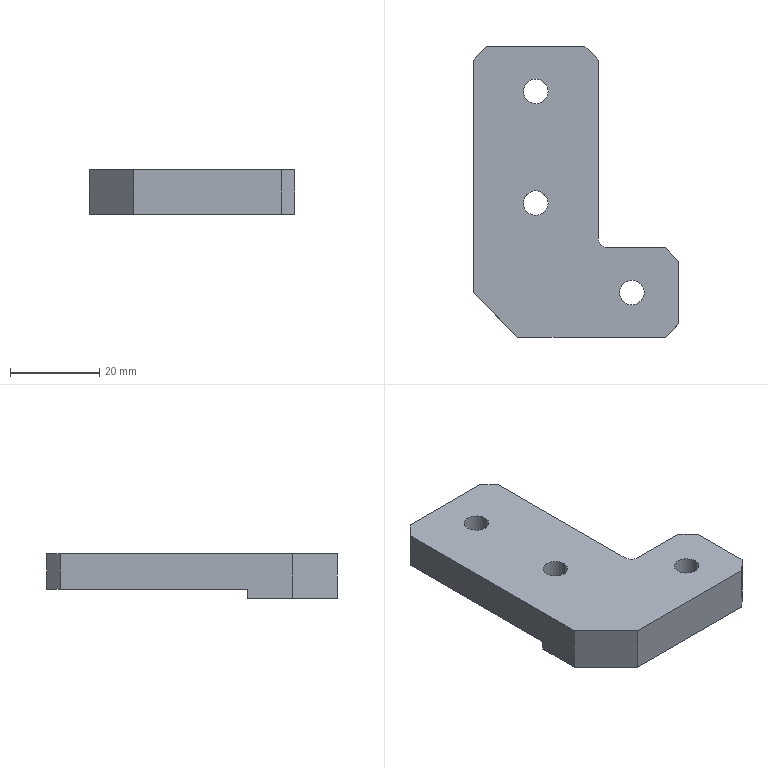Part | SolidWorks | features ICE 4, Chamfer 2, Extrusion 1, Fillet 1 | 1 solid | 21 faces | box 46 x 65 x 10 mm | volume 18007 mm3 | plane 14 | cylinder 7 | commonest cylinder face diameters 5.5 x6 4 x1
STEP:
#1=CARTESIAN_POINT('',(-34.75,30.,0.));
#2=VERTEX_POINT('',#1);
#3=CARTESIAN_POINT('',(-29.25,30.,0.));
#4=VERTEX_POINT('',#3);
#5=CARTESIAN_POINT('',(-32.,30.,0.));
#6=DIRECTION('',(0.,0.,1.));
#7=DIRECTION('',(1.,0.,0.));
#8=AXIS2_PLACEMENT_3D('',#5,#6,#7);
#9=CIRCLE('',#8,2.75);
#10=EDGE_CURVE('',#2,#4,#9,.T.);
#11=ORIENTED_EDGE('',*,*,#10,.F.);
#12=CARTESIAN_POINT('',(-34.75,30.,8.));
#13=VERTEX_POINT('',#12);
#14=CARTESIAN_POINT('',(-34.75,30.,-2.));
#15=DIRECTION('',(0.,0.,1.));
#16=VECTOR('',#15,1000.);
#17=LINE('',#14,#16);
#18=EDGE_CURVE('',#2,#13,#17,.T.);
#19=ORIENTED_EDGE('',*,*,#18,.T.);
#20=CARTESIAN_POINT('',(-29.25,30.,8.));
#21=VERTEX_POINT('',#20);
#22=CARTESIAN_POINT('',(-32.,30.,8.));
#23=DIRECTION('',(0.,0.,1.));
#24=DIRECTION('',(1.,0.,0.));
#25=AXIS2_PLACEMENT_3D('',#22,#23,#24);
#26=CIRCLE('',#25,2.75);
#27=EDGE_CURVE('',#13,#21,#26,.T.);
#28=ORIENTED_EDGE('',*,*,#27,.T.);
#29=CARTESIAN_POINT('',(-29.25,30.,-2.));
#30=DIRECTION('',(0.,0.,1.));
#31=VECTOR('',#30,1000.);
#32=LINE('',#29,#31);
#33=EDGE_CURVE('',#4,#21,#32,.T.);
#34=ORIENTED_EDGE('',*,*,#33,.F.);
#35=EDGE_LOOP('',(#11,#19,#28,#34));
#36=FACE_OUTER_BOUND('',#35,.T.);
#37=CARTESIAN_POINT('',(-32.,30.,-2.));
#38=DIRECTION('',(0.,0.,1.));
#39=DIRECTION('',(1.,0.,0.));
#40=AXIS2_PLACEMENT_3D('',#37,#38,#39);
#41=CYLINDRICAL_SURFACE('',#40,2.75);
#42=ADVANCED_FACE('',(#36),#41,.F.);
#43=CARTESIAN_POINT('',(-34.75,55.,0.));
#44=VERTEX_POINT('',#43);
#45=CARTESIAN_POINT('',(-29.25,55.,0.));
#46=VERTEX_POINT('',#45);
#47=CARTESIAN_POINT('',(-32.,55.,0.));
#48=DIRECTION('',(0.,0.,1.));
#49=DIRECTION('',(1.,0.,0.));
#50=AXIS2_PLACEMENT_3D('',#47,#48,#49);
#51=CIRCLE('',#50,2.75);
#52=EDGE_CURVE('',#44,#46,#51,.T.);
#53=ORIENTED_EDGE('',*,*,#52,.F.);
#54=CARTESIAN_POINT('',(-34.75,55.,8.));
#55=VERTEX_POINT('',#54);
#56=CARTESIAN_POINT('',(-34.75,55.,-2.));
#57=DIRECTION('',(0.,0.,1.));
#58=VECTOR('',#57,1000.);
#59=LINE('',#56,#58);
#60=EDGE_CURVE('',#44,#55,#59,.T.);
#61=ORIENTED_EDGE('',*,*,#60,.T.);
#62=CARTESIAN_POINT('',(-29.25,55.,8.));
#63=VERTEX_POINT('',#62);
#64=CARTESIAN_POINT('',(-32.,55.,8.));
#65=DIRECTION('',(0.,0.,1.));
#66=DIRECTION('',(1.,0.,0.));
#67=AXIS2_PLACEMENT_3D('',#64,#65,#66);
#68=CIRCLE('',#67,2.75);
#69=EDGE_CURVE('',#55,#63,#68,.T.);
#70=ORIENTED_EDGE('',*,*,#69,.T.);
#71=CARTESIAN_POINT('',(-29.25,55.,-2.));
#72=DIRECTION('',(0.,0.,1.));
#73=VECTOR('',#72,1000.);
#74=LINE('',#71,#73);
#75=EDGE_CURVE('',#46,#63,#74,.T.);
#76=ORIENTED_EDGE('',*,*,#75,.F.);
#77=EDGE_LOOP('',(#53,#61,#70,#76));
#78=FACE_OUTER_BOUND('',#77,.T.);
#79=CARTESIAN_POINT('',(-32.,55.,-2.));
#80=DIRECTION('',(0.,0.,1.));
#81=DIRECTION('',(1.,0.,0.));
#82=AXIS2_PLACEMENT_3D('',#79,#80,#81);
#83=CYLINDRICAL_SURFACE('',#82,2.75);
#84=ADVANCED_FACE('',(#78),#83,.F.);
#85=CARTESIAN_POINT('',(-7.75,10.,-2.));
#86=VERTEX_POINT('',#85);
#87=CARTESIAN_POINT('',(-13.25,10.,-2.));
#88=VERTEX_POINT('',#87);
#89=CARTESIAN_POINT('',(-10.5,10.,-2.));
#90=DIRECTION('',(0.,0.,-1.));
#91=DIRECTION('',(-1.,0.,0.));
#92=AXIS2_PLACEMENT_3D('',#89,#90,#91);
#93=CIRCLE('',#92,2.75);
#94=EDGE_CURVE('',#86,#88,#93,.T.);
#95=ORIENTED_EDGE('',*,*,#94,.T.);
#96=CARTESIAN_POINT('',(-13.25,10.,8.));
#97=VERTEX_POINT('',#96);
#98=CARTESIAN_POINT('',(-13.25,10.,-10.));
#99=DIRECTION('',(0.,0.,1.));
#100=VECTOR('',#99,1000.);
#101=LINE('',#98,#100);
#102=EDGE_CURVE('',#88,#97,#101,.T.);
#103=ORIENTED_EDGE('',*,*,#102,.T.);
#104=CARTESIAN_POINT('',(-7.75,10.,8.));
#105=VERTEX_POINT('',#104);
#106=CARTESIAN_POINT('',(-10.5,10.,8.));
#107=DIRECTION('',(0.,0.,1.));
#108=DIRECTION('',(1.,0.,0.));
#109=AXIS2_PLACEMENT_3D('',#106,#107,#108);
#110=CIRCLE('',#109,2.75);
#111=EDGE_CURVE('',#97,#105,#110,.T.);
#112=ORIENTED_EDGE('',*,*,#111,.T.);
#113=CARTESIAN_POINT('',(-7.75,10.,-10.));
#114=DIRECTION('',(0.,0.,1.));
#115=VECTOR('',#114,1000.);
#116=LINE('',#113,#115);
#117=EDGE_CURVE('',#86,#105,#116,.T.);
#118=ORIENTED_EDGE('',*,*,#117,.F.);
#119=EDGE_LOOP('',(#95,#103,#112,#118));
#120=FACE_OUTER_BOUND('',#119,.T.);
#121=CARTESIAN_POINT('',(-10.5,10.,-10.));
#122=DIRECTION('',(0.,0.,1.));
#123=DIRECTION('',(1.,0.,0.));
#124=AXIS2_PLACEMENT_3D('',#121,#122,#123);
#125=CYLINDRICAL_SURFACE('',#124,2.75);
#126=ADVANCED_FACE('',(#120),#125,.F.);
#127=CARTESIAN_POINT('',(-32.,55.,0.));
#128=DIRECTION('',(0.,0.,1.));
#129=DIRECTION('',(1.,0.,0.));
#130=AXIS2_PLACEMENT_3D('',#127,#128,#129);
#131=CIRCLE('',#130,2.75);
#132=EDGE_CURVE('',#46,#44,#131,.T.);
#133=ORIENTED_EDGE('',*,*,#132,.T.);
#134=ORIENTED_EDGE('',*,*,#52,.T.);
#135=EDGE_LOOP('',(#133,#134));
#136=FACE_BOUND('',#135,.T.);
#137=CARTESIAN_POINT('',(-32.,30.,0.));
#138=DIRECTION('',(0.,0.,1.));
#139=DIRECTION('',(1.,0.,0.));
#140=AXIS2_PLACEMENT_3D('',#137,#138,#139);
#141=CIRCLE('',#140,2.75);
#142=EDGE_CURVE('',#4,#2,#141,.T.);
#143=ORIENTED_EDGE('',*,*,#142,.T.);
#144=ORIENTED_EDGE('',*,*,#10,.T.);
#145=EDGE_LOOP('',(#143,#144));
#146=FACE_BOUND('',#145,.T.);
#147=CARTESIAN_POINT('',(-21.,65.,0.));
#148=VERTEX_POINT('',#147);
#149=CARTESIAN_POINT('',(-43.,65.,0.));
#150=VERTEX_POINT('',#149);
#151=CARTESIAN_POINT('',(0.,65.,0.));
#152=DIRECTION('',(-1.,0.,0.));
#153=VECTOR('',#152,1000.);
#154=LINE('',#151,#153);
#155=EDGE_CURVE('',#148,#150,#154,.T.);
#156=ORIENTED_EDGE('',*,*,#155,.F.);
#157=CARTESIAN_POINT('',(-18.,62.,0.));
#158=VERTEX_POINT('',#157);
#159=CARTESIAN_POINT('',(-18.,62.,0.));
#160=DIRECTION('',(0.7071,-0.7071,0.));
#161=VECTOR('',#160,1000.);
#162=LINE('',#159,#161);
#163=EDGE_CURVE('',#148,#158,#162,.T.);
#164=ORIENTED_EDGE('',*,*,#163,.T.);
#165=CARTESIAN_POINT('',(-18.,22.,0.));
#166=VERTEX_POINT('',#165);
#167=CARTESIAN_POINT('',(-18.,0.,0.));
#168=DIRECTION('',(0.,-1.,0.));
#169=VECTOR('',#168,1000.);
#170=LINE('',#167,#169);
#171=EDGE_CURVE('',#158,#166,#170,.T.);
#172=ORIENTED_EDGE('',*,*,#171,.T.);
#173=CARTESIAN_POINT('',(-16.,20.,0.));
#174=VERTEX_POINT('',#173);
#175=CARTESIAN_POINT('',(-16.,22.,0.));
#176=DIRECTION('',(0.,0.,1.));
#177=DIRECTION('',(1.,0.,0.));
#178=AXIS2_PLACEMENT_3D('',#175,#176,#177);
#179=CIRCLE('',#178,2.);
#180=EDGE_CURVE('',#166,#174,#179,.T.);
#181=ORIENTED_EDGE('',*,*,#180,.T.);
#182=CARTESIAN_POINT('',(-46.,20.,0.));
#183=VERTEX_POINT('',#182);
#184=CARTESIAN_POINT('',(0.,20.,0.));
#185=DIRECTION('',(1.,0.,0.));
#186=VECTOR('',#185,1000.);
#187=LINE('',#184,#186);
#188=EDGE_CURVE('',#183,#174,#187,.T.);
#189=ORIENTED_EDGE('',*,*,#188,.F.);
#190=CARTESIAN_POINT('',(-46.,62.,0.));
#191=VERTEX_POINT('',#190);
#192=CARTESIAN_POINT('',(-46.,0.,0.));
#193=DIRECTION('',(0.,-1.,0.));
#194=VECTOR('',#193,1000.);
#195=LINE('',#192,#194);
#196=EDGE_CURVE('',#191,#183,#195,.T.);
#197=ORIENTED_EDGE('',*,*,#196,.F.);
#198=CARTESIAN_POINT('',(-46.,62.,0.));
#199=DIRECTION('',(0.7071,0.7071,0.));
#200=VECTOR('',#199,1000.);
#201=LINE('',#198,#200);
#202=EDGE_CURVE('',#191,#150,#201,.T.);
#203=ORIENTED_EDGE('',*,*,#202,.T.);
#204=EDGE_LOOP('',(#156,#164,#172,#181,#189,#197,#203));
#205=FACE_OUTER_BOUND('',#204,.T.);
#206=CARTESIAN_POINT('',(0.,0.,0.));
#207=DIRECTION('',(0.,0.,1.));
#208=DIRECTION('',(1.,0.,0.));
#209=AXIS2_PLACEMENT_3D('',#206,#207,#208);
#210=PLANE('',#209);
#211=ADVANCED_FACE('',(#136,#146,#205),#210,.F.);
#212=CARTESIAN_POINT('',(0.,3.,8.));
#213=VERTEX_POINT('',#212);
#214=CARTESIAN_POINT('',(0.,17.,8.));
#215=VERTEX_POINT('',#214);
#216=CARTESIAN_POINT('',(0.,0.,8.));
#217=DIRECTION('',(0.,1.,0.));
#218=VECTOR('',#217,1000.);
#219=LINE('',#216,#218);
#220=EDGE_CURVE('',#213,#215,#219,.T.);
#221=ORIENTED_EDGE('',*,*,#220,.F.);
#222=CARTESIAN_POINT('',(0.,3.,-2.));
#223=VERTEX_POINT('',#222);
#224=CARTESIAN_POINT('',(0.,3.,8.));
#225=DIRECTION('',(0.,0.,-1.));
#226=VECTOR('',#225,1000.);
#227=LINE('',#224,#226);
#228=EDGE_CURVE('',#213,#223,#227,.T.);
#229=ORIENTED_EDGE('',*,*,#228,.T.);
#230=CARTESIAN_POINT('',(0.,17.,-2.));
#231=VERTEX_POINT('',#230);
#232=CARTESIAN_POINT('',(0.,20.,-2.));
#233=DIRECTION('',(0.,-1.,0.));
#234=VECTOR('',#233,1000.);
#235=LINE('',#232,#234);
#236=EDGE_CURVE('',#231,#223,#235,.T.);
#237=ORIENTED_EDGE('',*,*,#236,.F.);
#238=CARTESIAN_POINT('',(0.,17.,8.));
#239=DIRECTION('',(0.,0.,1.));
#240=VECTOR('',#239,1000.);
#241=LINE('',#238,#240);
#242=EDGE_CURVE('',#231,#215,#241,.T.);
#243=ORIENTED_EDGE('',*,*,#242,.T.);
#244=EDGE_LOOP('',(#221,#229,#237,#243));
#245=FACE_OUTER_BOUND('',#244,.T.);
#246=CARTESIAN_POINT('',(0.,0.,8.));
#247=DIRECTION('',(-1.,0.,0.));
#248=DIRECTION('',(0.,0.,1.));
#249=AXIS2_PLACEMENT_3D('',#246,#247,#248);
#250=PLANE('',#249);
#251=ADVANCED_FACE('',(#245),#250,.F.);
#252=CARTESIAN_POINT('',(-21.,65.,8.));
#253=VERTEX_POINT('',#252);
#254=CARTESIAN_POINT('',(-43.,65.,8.));
#255=VERTEX_POINT('',#254);
#256=CARTESIAN_POINT('',(0.,65.,8.));
#257=DIRECTION('',(-1.,0.,0.));
#258=VECTOR('',#257,1000.);
#259=LINE('',#256,#258);
#260=EDGE_CURVE('',#253,#255,#259,.T.);
#261=ORIENTED_EDGE('',*,*,#260,.F.);
#262=CARTESIAN_POINT('',(-21.,65.,8.));
#263=DIRECTION('',(0.,0.,-1.));
#264=VECTOR('',#263,1000.);
#265=LINE('',#262,#264);
#266=EDGE_CURVE('',#253,#148,#265,.T.);
#267=ORIENTED_EDGE('',*,*,#266,.T.);
#268=ORIENTED_EDGE('',*,*,#155,.T.);
#269=CARTESIAN_POINT('',(-43.,65.,8.));
#270=DIRECTION('',(0.,0.,1.));
#271=VECTOR('',#270,1000.);
#272=LINE('',#269,#271);
#273=EDGE_CURVE('',#150,#255,#272,.T.);
#274=ORIENTED_EDGE('',*,*,#273,.T.);
#275=EDGE_LOOP('',(#261,#267,#268,#274));
#276=FACE_OUTER_BOUND('',#275,.T.);
#277=CARTESIAN_POINT('',(0.,65.,8.));
#278=DIRECTION('',(0.,-1.,0.));
#279=DIRECTION('',(0.,0.,-1.));
#280=AXIS2_PLACEMENT_3D('',#277,#278,#279);
#281=PLANE('',#280);
#282=ADVANCED_FACE('',(#276),#281,.F.);
#283=CARTESIAN_POINT('',(-46.,62.,8.));
#284=VERTEX_POINT('',#283);
#285=CARTESIAN_POINT('',(-46.,10.,8.));
#286=VERTEX_POINT('',#285);
#287=CARTESIAN_POINT('',(-46.,0.,8.));
#288=DIRECTION('',(0.,-1.,0.));
#289=VECTOR('',#288,1000.);
#290=LINE('',#287,#289);
#291=EDGE_CURVE('',#284,#286,#290,.T.);
#292=ORIENTED_EDGE('',*,*,#291,.F.);
#293=CARTESIAN_POINT('',(-46.,62.,8.));
#294=DIRECTION('',(0.,0.,-1.));
#295=VECTOR('',#294,1000.);
#296=LINE('',#293,#295);
#297=EDGE_CURVE('',#284,#191,#296,.T.);
#298=ORIENTED_EDGE('',*,*,#297,.T.);
#299=ORIENTED_EDGE('',*,*,#196,.T.);
#300=CARTESIAN_POINT('',(-46.,20.,-2.));
#301=VERTEX_POINT('',#300);
#302=CARTESIAN_POINT('',(-46.,20.,-2.));
#303=DIRECTION('',(0.,0.,1.));
#304=VECTOR('',#303,1000.);
#305=LINE('',#302,#304);
#306=EDGE_CURVE('',#301,#183,#305,.T.);
#307=ORIENTED_EDGE('',*,*,#306,.F.);
#308=CARTESIAN_POINT('',(-46.,10.,-2.));
#309=VERTEX_POINT('',#308);
#310=CARTESIAN_POINT('',(-46.,20.,-2.));
#311=DIRECTION('',(0.,1.,0.));
#312=VECTOR('',#311,1000.);
#313=LINE('',#310,#312);
#314=EDGE_CURVE('',#309,#301,#313,.T.);
#315=ORIENTED_EDGE('',*,*,#314,.F.);
#316=CARTESIAN_POINT('',(-46.,10.,8.));
#317=DIRECTION('',(0.,0.,1.));
#318=VECTOR('',#317,1000.);
#319=LINE('',#316,#318);
#320=EDGE_CURVE('',#309,#286,#319,.T.);
#321=ORIENTED_EDGE('',*,*,#320,.T.);
#322=EDGE_LOOP('',(#292,#298,#299,#307,#315,#321));
#323=FACE_OUTER_BOUND('',#322,.T.);
#324=CARTESIAN_POINT('',(-46.,0.,8.));
#325=DIRECTION('',(1.,0.,0.));
#326=DIRECTION('',(0.,0.,-1.));
#327=AXIS2_PLACEMENT_3D('',#324,#325,#326);
#328=PLANE('',#327);
#329=ADVANCED_FACE('',(#323),#328,.F.);
#330=CARTESIAN_POINT('',(-3.,0.,-2.));
#331=VERTEX_POINT('',#330);
#332=CARTESIAN_POINT('',(-36.,0.,-2.));
#333=VERTEX_POINT('',#332);
#334=CARTESIAN_POINT('',(-36.,0.,-2.));
#335=DIRECTION('',(-1.,0.,0.));
#336=VECTOR('',#335,1000.);
#337=LINE('',#334,#336);
#338=EDGE_CURVE('',#331,#333,#337,.T.);
#339=ORIENTED_EDGE('',*,*,#338,.F.);
#340=CARTESIAN_POINT('',(-3.,0.,8.));
#341=VERTEX_POINT('',#340);
#342=CARTESIAN_POINT('',(-3.,0.,8.));
#343=DIRECTION('',(0.,0.,1.));
#344=VECTOR('',#343,1000.);
#345=LINE('',#342,#344);
#346=EDGE_CURVE('',#331,#341,#345,.T.);
#347=ORIENTED_EDGE('',*,*,#346,.T.);
#348=CARTESIAN_POINT('',(-36.,0.,8.));
#349=VERTEX_POINT('',#348);
#350=CARTESIAN_POINT('',(0.,0.,8.));
#351=DIRECTION('',(1.,0.,0.));
#352=VECTOR('',#351,1000.);
#353=LINE('',#350,#352);
#354=EDGE_CURVE('',#349,#341,#353,.T.);
#355=ORIENTED_EDGE('',*,*,#354,.F.);
#356=CARTESIAN_POINT('',(-36.,0.,8.));
#357=DIRECTION('',(0.,0.,-1.));
#358=VECTOR('',#357,1000.);
#359=LINE('',#356,#358);
#360=EDGE_CURVE('',#349,#333,#359,.T.);
#361=ORIENTED_EDGE('',*,*,#360,.T.);
#362=EDGE_LOOP('',(#339,#347,#355,#361));
#363=FACE_OUTER_BOUND('',#362,.T.);
#364=CARTESIAN_POINT('',(0.,0.,8.));
#365=DIRECTION('',(0.,1.,0.));
#366=DIRECTION('',(-1.,0.,0.));
#367=AXIS2_PLACEMENT_3D('',#364,#365,#366);
#368=PLANE('',#367);
#369=ADVANCED_FACE('',(#363),#368,.F.);
#370=ORIENTED_EDGE('',*,*,#354,.T.);
#371=CARTESIAN_POINT('',(-1.5,1.5,8.));
#372=DIRECTION('',(0.7071,0.7071,0.));
#373=VECTOR('',#372,1000.);
#374=LINE('',#371,#373);
#375=EDGE_CURVE('',#341,#213,#374,.T.);
#376=ORIENTED_EDGE('',*,*,#375,.T.);
#377=ORIENTED_EDGE('',*,*,#220,.T.);
#378=CARTESIAN_POINT('',(-3.,20.,8.));
#379=VERTEX_POINT('',#378);
#380=CARTESIAN_POINT('',(8.5,8.5,8.));
#381=DIRECTION('',(-0.7071,0.7071,0.));
#382=VECTOR('',#381,1000.);
#383=LINE('',#380,#382);
#384=EDGE_CURVE('',#215,#379,#383,.T.);
#385=ORIENTED_EDGE('',*,*,#384,.T.);
#386=CARTESIAN_POINT('',(-16.,20.,8.));
#387=VERTEX_POINT('',#386);
#388=CARTESIAN_POINT('',(0.,20.,8.));
#389=DIRECTION('',(1.,0.,0.));
#390=VECTOR('',#389,1000.);
#391=LINE('',#388,#390);
#392=EDGE_CURVE('',#387,#379,#391,.T.);
#393=ORIENTED_EDGE('',*,*,#392,.F.);
#394=CARTESIAN_POINT('',(-18.,22.,8.));
#395=VERTEX_POINT('',#394);
#396=CARTESIAN_POINT('',(-16.,22.,8.));
#397=DIRECTION('',(0.,0.,-1.));
#398=DIRECTION('',(1.,0.,0.));
#399=AXIS2_PLACEMENT_3D('',#396,#397,#398);
#400=CIRCLE('',#399,2.);
#401=EDGE_CURVE('',#387,#395,#400,.T.);
#402=ORIENTED_EDGE('',*,*,#401,.T.);
#403=CARTESIAN_POINT('',(-18.,62.,8.));
#404=VERTEX_POINT('',#403);
#405=CARTESIAN_POINT('',(-18.,65.,8.));
#406=DIRECTION('',(0.,-1.,0.));
#407=VECTOR('',#406,1000.);
#408=LINE('',#405,#407);
#409=EDGE_CURVE('',#404,#395,#408,.T.);
#410=ORIENTED_EDGE('',*,*,#409,.F.);
#411=CARTESIAN_POINT('',(22.,22.,8.));
#412=DIRECTION('',(-0.7071,0.7071,0.));
#413=VECTOR('',#412,1000.);
#414=LINE('',#411,#413);
#415=EDGE_CURVE('',#404,#253,#414,.T.);
#416=ORIENTED_EDGE('',*,*,#415,.T.);
#417=ORIENTED_EDGE('',*,*,#260,.T.);
#418=CARTESIAN_POINT('',(-54.,54.,8.));
#419=DIRECTION('',(-0.7071,-0.7071,0.));
#420=VECTOR('',#419,1000.);
#421=LINE('',#418,#420);
#422=EDGE_CURVE('',#255,#284,#421,.T.);
#423=ORIENTED_EDGE('',*,*,#422,.T.);
#424=ORIENTED_EDGE('',*,*,#291,.T.);
#425=CARTESIAN_POINT('',(-18.,-18.,8.));
#426=DIRECTION('',(0.7071,-0.7071,0.));
#427=VECTOR('',#426,1000.);
#428=LINE('',#425,#427);
#429=EDGE_CURVE('',#286,#349,#428,.T.);
#430=ORIENTED_EDGE('',*,*,#429,.T.);
#431=EDGE_LOOP('',(#370,#376,#377,#385,#393,#402,#410,#416,#417,#423,#424,#430));
#432=FACE_OUTER_BOUND('',#431,.T.);
#433=CARTESIAN_POINT('',(-32.,30.,8.));
#434=DIRECTION('',(0.,0.,1.));
#435=DIRECTION('',(1.,0.,0.));
#436=AXIS2_PLACEMENT_3D('',#433,#434,#435);
#437=CIRCLE('',#436,2.75);
#438=EDGE_CURVE('',#21,#13,#437,.T.);
#439=ORIENTED_EDGE('',*,*,#438,.F.);
#440=ORIENTED_EDGE('',*,*,#27,.F.);
#441=EDGE_LOOP('',(#439,#440));
#442=FACE_BOUND('',#441,.T.);
#443=CARTESIAN_POINT('',(-32.,55.,8.));
#444=DIRECTION('',(0.,0.,1.));
#445=DIRECTION('',(1.,0.,0.));
#446=AXIS2_PLACEMENT_3D('',#443,#444,#445);
#447=CIRCLE('',#446,2.75);
#448=EDGE_CURVE('',#63,#55,#447,.T.);
#449=ORIENTED_EDGE('',*,*,#448,.F.);
#450=ORIENTED_EDGE('',*,*,#69,.F.);
#451=EDGE_LOOP('',(#449,#450));
#452=FACE_BOUND('',#451,.T.);
#453=CARTESIAN_POINT('',(-10.5,10.,8.));
#454=DIRECTION('',(0.,0.,1.));
#455=DIRECTION('',(1.,0.,0.));
#456=AXIS2_PLACEMENT_3D('',#453,#454,#455);
#457=CIRCLE('',#456,2.75);
#458=EDGE_CURVE('',#105,#97,#457,.T.);
#459=ORIENTED_EDGE('',*,*,#458,.F.);
#460=ORIENTED_EDGE('',*,*,#111,.F.);
#461=EDGE_LOOP('',(#459,#460));
#462=FACE_BOUND('',#461,.T.);
#463=CARTESIAN_POINT('',(0.,0.,8.));
#464=DIRECTION('',(0.,0.,1.));
#465=DIRECTION('',(1.,0.,0.));
#466=AXIS2_PLACEMENT_3D('',#463,#464,#465);
#467=PLANE('',#466);
#468=ADVANCED_FACE('',(#432,#442,#452,#462),#467,.T.);
#469=ORIENTED_EDGE('',*,*,#102,.F.);
#470=CARTESIAN_POINT('',(-10.5,10.,-2.));
#471=DIRECTION('',(0.,0.,-1.));
#472=DIRECTION('',(-1.,0.,0.));
#473=AXIS2_PLACEMENT_3D('',#470,#471,#472);
#474=CIRCLE('',#473,2.75);
#475=EDGE_CURVE('',#88,#86,#474,.T.);
#476=ORIENTED_EDGE('',*,*,#475,.T.);
#477=ORIENTED_EDGE('',*,*,#117,.T.);
#478=ORIENTED_EDGE('',*,*,#458,.T.);
#479=EDGE_LOOP('',(#469,#476,#477,#478));
#480=FACE_OUTER_BOUND('',#479,.T.);
#481=CARTESIAN_POINT('',(-10.5,10.,-10.));
#482=DIRECTION('',(0.,0.,1.));
#483=DIRECTION('',(1.,0.,0.));
#484=AXIS2_PLACEMENT_3D('',#481,#482,#483);
#485=CYLINDRICAL_SURFACE('',#484,2.75);
#486=ADVANCED_FACE('',(#480),#485,.F.);
#487=ORIENTED_EDGE('',*,*,#429,.F.);
#488=ORIENTED_EDGE('',*,*,#320,.F.);
#489=CARTESIAN_POINT('',(-36.,0.,-2.));
#490=DIRECTION('',(-0.7071,0.7071,0.));
#491=VECTOR('',#490,1000.);
#492=LINE('',#489,#491);
#493=EDGE_CURVE('',#333,#309,#492,.T.);
#494=ORIENTED_EDGE('',*,*,#493,.F.);
#495=ORIENTED_EDGE('',*,*,#360,.F.);
#496=EDGE_LOOP('',(#487,#488,#494,#495));
#497=FACE_OUTER_BOUND('',#496,.T.);
#498=CARTESIAN_POINT('',(-36.,0.,8.));
#499=DIRECTION('',(0.7071,0.7071,0.));
#500=DIRECTION('',(0.,0.,-1.));
#501=AXIS2_PLACEMENT_3D('',#498,#499,#500);
#502=PLANE('',#501);
#503=ADVANCED_FACE('',(#497),#502,.F.);
#504=ORIENTED_EDGE('',*,*,#60,.F.);
#505=ORIENTED_EDGE('',*,*,#132,.F.);
#506=ORIENTED_EDGE('',*,*,#75,.T.);
#507=ORIENTED_EDGE('',*,*,#448,.T.);
#508=EDGE_LOOP('',(#504,#505,#506,#507));
#509=FACE_OUTER_BOUND('',#508,.T.);
#510=CARTESIAN_POINT('',(-32.,55.,-2.));
#511=DIRECTION('',(0.,0.,1.));
#512=DIRECTION('',(1.,0.,0.));
#513=AXIS2_PLACEMENT_3D('',#510,#511,#512);
#514=CYLINDRICAL_SURFACE('',#513,2.75);
#515=ADVANCED_FACE('',(#509),#514,.F.);
#516=ORIENTED_EDGE('',*,*,#18,.F.);
#517=ORIENTED_EDGE('',*,*,#142,.F.);
#518=ORIENTED_EDGE('',*,*,#33,.T.);
#519=ORIENTED_EDGE('',*,*,#438,.T.);
#520=EDGE_LOOP('',(#516,#517,#518,#519));
#521=FACE_OUTER_BOUND('',#520,.T.);
#522=CARTESIAN_POINT('',(-32.,30.,-2.));
#523=DIRECTION('',(0.,0.,1.));
#524=DIRECTION('',(1.,0.,0.));
#525=AXIS2_PLACEMENT_3D('',#522,#523,#524);
#526=CYLINDRICAL_SURFACE('',#525,2.75);
#527=ADVANCED_FACE('',(#521),#526,.F.);
#528=ORIENTED_EDGE('',*,*,#392,.T.);
#529=CARTESIAN_POINT('',(-3.,20.,-2.));
#530=VERTEX_POINT('',#529);
#531=CARTESIAN_POINT('',(-3.,20.,-2.));
#532=DIRECTION('',(0.,0.,-1.));
#533=VECTOR('',#532,1000.);
#534=LINE('',#531,#533);
#535=EDGE_CURVE('',#379,#530,#534,.T.);
#536=ORIENTED_EDGE('',*,*,#535,.T.);
#537=CARTESIAN_POINT('',(0.,20.,-2.));
#538=DIRECTION('',(1.,0.,0.));
#539=VECTOR('',#538,1000.);
#540=LINE('',#537,#539);
#541=EDGE_CURVE('',#301,#530,#540,.T.);
#542=ORIENTED_EDGE('',*,*,#541,.F.);
#543=ORIENTED_EDGE('',*,*,#306,.T.);
#544=ORIENTED_EDGE('',*,*,#188,.T.);
#545=CARTESIAN_POINT('',(-16.,20.,8.));
#546=DIRECTION('',(0.,0.,1.));
#547=VECTOR('',#546,1000.);
#548=LINE('',#545,#547);
#549=EDGE_CURVE('',#174,#387,#548,.T.);
#550=ORIENTED_EDGE('',*,*,#549,.T.);
#551=EDGE_LOOP('',(#528,#536,#542,#543,#544,#550));
#552=FACE_OUTER_BOUND('',#551,.T.);
#553=CARTESIAN_POINT('',(0.,20.,-2.));
#554=DIRECTION('',(0.,-1.,0.));
#555=DIRECTION('',(1.,0.,0.));
#556=AXIS2_PLACEMENT_3D('',#553,#554,#555);
#557=PLANE('',#556);
#558=ADVANCED_FACE('',(#552),#557,.F.);
#559=ORIENTED_EDGE('',*,*,#171,.F.);
#560=CARTESIAN_POINT('',(-18.,62.,-2.));
#561=DIRECTION('',(0.,0.,1.));
#562=VECTOR('',#561,1000.);
#563=LINE('',#560,#562);
#564=EDGE_CURVE('',#158,#404,#563,.T.);
#565=ORIENTED_EDGE('',*,*,#564,.T.);
#566=ORIENTED_EDGE('',*,*,#409,.T.);
#567=CARTESIAN_POINT('',(-18.,22.,0.));
#568=DIRECTION('',(0.,0.,-1.));
#569=VECTOR('',#568,1000.);
#570=LINE('',#567,#569);
#571=EDGE_CURVE('',#395,#166,#570,.T.);
#572=ORIENTED_EDGE('',*,*,#571,.T.);
#573=EDGE_LOOP('',(#559,#565,#566,#572));
#574=FACE_OUTER_BOUND('',#573,.T.);
#575=CARTESIAN_POINT('',(-18.,65.,-2.));
#576=DIRECTION('',(-1.,0.,0.));
#577=DIRECTION('',(0.,-1.,0.));
#578=AXIS2_PLACEMENT_3D('',#575,#576,#577);
#579=PLANE('',#578);
#580=ADVANCED_FACE('',(#574),#579,.F.);
#581=ORIENTED_EDGE('',*,*,#236,.T.);
#582=CARTESIAN_POINT('',(0.,3.,-2.));
#583=DIRECTION('',(-0.7071,-0.7071,0.));
#584=VECTOR('',#583,1000.);
#585=LINE('',#582,#584);
#586=EDGE_CURVE('',#223,#331,#585,.T.);
#587=ORIENTED_EDGE('',*,*,#586,.T.);
#588=ORIENTED_EDGE('',*,*,#338,.T.);
#589=ORIENTED_EDGE('',*,*,#493,.T.);
#590=ORIENTED_EDGE('',*,*,#314,.T.);
#591=ORIENTED_EDGE('',*,*,#541,.T.);
#592=CARTESIAN_POINT('',(0.,17.,-2.));
#593=DIRECTION('',(0.7071,-0.7071,0.));
#594=VECTOR('',#593,1000.);
#595=LINE('',#592,#594);
#596=EDGE_CURVE('',#530,#231,#595,.T.);
#597=ORIENTED_EDGE('',*,*,#596,.T.);
#598=EDGE_LOOP('',(#581,#587,#588,#589,#590,#591,#597));
#599=FACE_OUTER_BOUND('',#598,.T.);
#600=ORIENTED_EDGE('',*,*,#94,.F.);
#601=ORIENTED_EDGE('',*,*,#475,.F.);
#602=EDGE_LOOP('',(#600,#601));
#603=FACE_BOUND('',#602,.T.);
#604=CARTESIAN_POINT('',(0.,0.,-2.));
#605=DIRECTION('',(0.,0.,1.));
#606=DIRECTION('',(1.,0.,0.));
#607=AXIS2_PLACEMENT_3D('',#604,#605,#606);
#608=PLANE('',#607);
#609=ADVANCED_FACE('',(#599,#603),#608,.F.);
#610=ORIENTED_EDGE('',*,*,#180,.F.);
#611=ORIENTED_EDGE('',*,*,#571,.F.);
#612=ORIENTED_EDGE('',*,*,#401,.F.);
#613=ORIENTED_EDGE('',*,*,#549,.F.);
#614=EDGE_LOOP('',(#610,#611,#612,#613));
#615=FACE_OUTER_BOUND('',#614,.T.);
#616=CARTESIAN_POINT('',(-16.,22.,-2.));
#617=DIRECTION('',(0.,0.,-1.));
#618=DIRECTION('',(-1.,0.,0.));
#619=AXIS2_PLACEMENT_3D('',#616,#617,#618);
#620=CYLINDRICAL_SURFACE('',#619,2.);
#621=ADVANCED_FACE('',(#615),#620,.F.);
#622=ORIENTED_EDGE('',*,*,#375,.F.);
#623=ORIENTED_EDGE('',*,*,#346,.F.);
#624=ORIENTED_EDGE('',*,*,#586,.F.);
#625=ORIENTED_EDGE('',*,*,#228,.F.);
#626=EDGE_LOOP('',(#622,#623,#624,#625));
#627=FACE_OUTER_BOUND('',#626,.T.);
#628=CARTESIAN_POINT('',(0.,3.,8.));
#629=DIRECTION('',(-0.7071,0.7071,0.));
#630=DIRECTION('',(0.,0.,-1.));
#631=AXIS2_PLACEMENT_3D('',#628,#629,#630);
#632=PLANE('',#631);
#633=ADVANCED_FACE('',(#627),#632,.F.);
#634=ORIENTED_EDGE('',*,*,#596,.F.);
#635=ORIENTED_EDGE('',*,*,#535,.F.);
#636=ORIENTED_EDGE('',*,*,#384,.F.);
#637=ORIENTED_EDGE('',*,*,#242,.F.);
#638=EDGE_LOOP('',(#634,#635,#636,#637));
#639=FACE_OUTER_BOUND('',#638,.T.);
#640=CARTESIAN_POINT('',(0.,17.,8.));
#641=DIRECTION('',(-0.7071,-0.7071,0.));
#642=DIRECTION('',(0.,0.,1.));
#643=AXIS2_PLACEMENT_3D('',#640,#641,#642);
#644=PLANE('',#643);
#645=ADVANCED_FACE('',(#639),#644,.F.);
#646=ORIENTED_EDGE('',*,*,#163,.F.);
#647=ORIENTED_EDGE('',*,*,#266,.F.);
#648=ORIENTED_EDGE('',*,*,#415,.F.);
#649=ORIENTED_EDGE('',*,*,#564,.F.);
#650=EDGE_LOOP('',(#646,#647,#648,#649));
#651=FACE_OUTER_BOUND('',#650,.T.);
#652=CARTESIAN_POINT('',(-18.,62.,-2.));
#653=DIRECTION('',(-0.7071,-0.7071,0.));
#654=DIRECTION('',(0.,0.,1.));
#655=AXIS2_PLACEMENT_3D('',#652,#653,#654);
#656=PLANE('',#655);
#657=ADVANCED_FACE('',(#651),#656,.F.);
#658=ORIENTED_EDGE('',*,*,#422,.F.);
#659=ORIENTED_EDGE('',*,*,#273,.F.);
#660=ORIENTED_EDGE('',*,*,#202,.F.);
#661=ORIENTED_EDGE('',*,*,#297,.F.);
#662=EDGE_LOOP('',(#658,#659,#660,#661));
#663=FACE_OUTER_BOUND('',#662,.T.);
#664=CARTESIAN_POINT('',(-46.,62.,8.));
#665=DIRECTION('',(0.7071,-0.7071,0.));
#666=DIRECTION('',(0.,0.,-1.));
#667=AXIS2_PLACEMENT_3D('',#664,#665,#666);
#668=PLANE('',#667);
#669=ADVANCED_FACE('',(#663),#668,.F.);
#670=CLOSED_SHELL('',(#42,#84,#126,#211,#251,#282,#329,#369,#468,#486,#503,#515,#527,#558,#580,#609,#621,#633,#645,#657,#669));
#671=MANIFOLD_SOLID_BREP('',#670);
#672=CARTESIAN_POINT('',(0.,0.,0.));
#673=DIRECTION('',(0.,0.,1.));
#674=DIRECTION('',(1.,0.,0.));
#675=AXIS2_PLACEMENT_3D('',#672,#673,#674);
#676=(LENGTH_UNIT()NAMED_UNIT(*)SI_UNIT(.MILLI.,.METRE.));
#677=UNCERTAINTY_MEASURE_WITH_UNIT(LENGTH_MEASURE(0.00001),#676,'','');
#678=(NAMED_UNIT(*)PLANE_ANGLE_UNIT()SI_UNIT($,.RADIAN.));
#679=(NAMED_UNIT(*)SI_UNIT($,.STERADIAN.)SOLID_ANGLE_UNIT());
#680=(GEOMETRIC_REPRESENTATION_CONTEXT(3)GLOBAL_UNCERTAINTY_ASSIGNED_CONTEXT((#677))GLOBAL_UNIT_ASSIGNED_CONTEXT((#676,#678,#679))REPRESENTATION_CONTEXT('',''));
#681=ADVANCED_BREP_SHAPE_REPRESENTATION('',(#671,#675),#680);